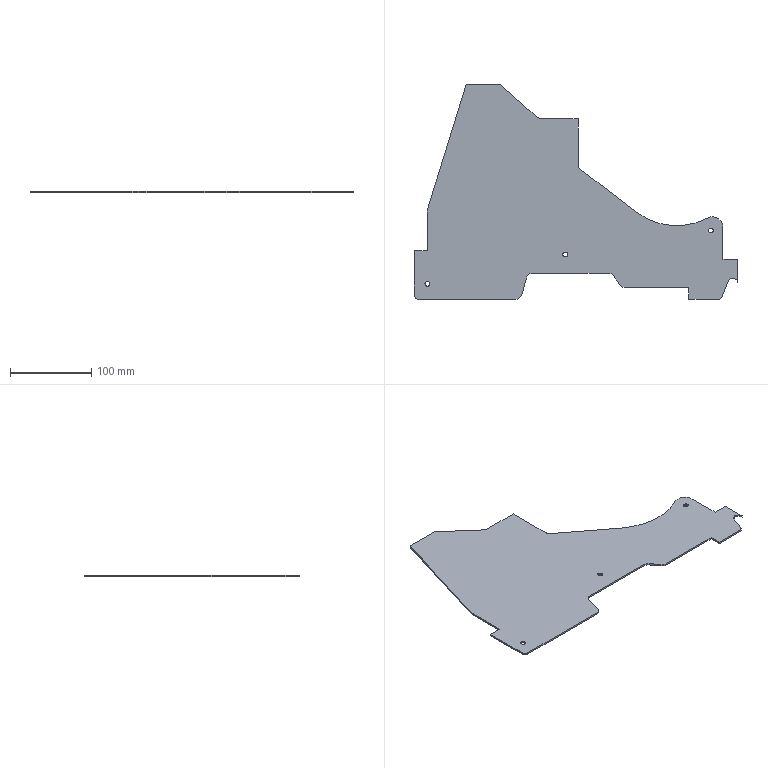Part | STEP file | 1 solid | 38 faces | box 398.474 x 264.335 x 2 mm | volume 117575 mm3 | plane 22 | cylinder 16 | commonest cylinder face diameters 6 x6 16 x4 10 x3 12 x1 25.909 x1 162.284 x1